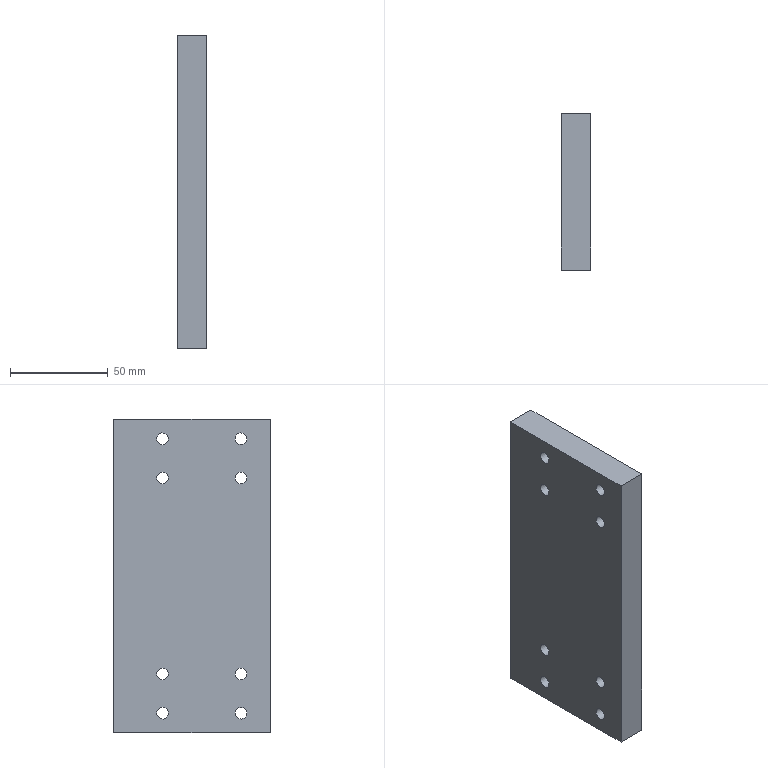Part | STEP file | SN10_008_007-01_PLACA | 1 solid | 14 faces | box 15 x 80 x 160 mm | volume 188607 mm3 | cylinder 8 | plane 6 | commonest cylinder face diameters 6 x8
STEP:
#1=CARTESIAN_POINT('',(0.,0.,0.));
#2=DIRECTION('',(0.,0.,1.));
#3=DIRECTION('',(1.,0.,0.));
#4=AXIS2_PLACEMENT_3D('',#1,#2,#3);
#5=CARTESIAN_POINT('',(308.629,177.633,427.708));
#6=VERTEX_POINT('',#5);
#7=CARTESIAN_POINT('',(308.629,175.,426.27));
#8=DIRECTION('',(1.,0.,0.));
#9=DIRECTION('',(0.,1.,0.));
#10=AXIS2_PLACEMENT_3D('',#7,#8,#9);
#11=CIRCLE('',#10,3.);
#12=CARTESIAN_POINT('',(308.729,175.,426.27));
#13=DIRECTION('',(1.,0.,0.));
#14=DIRECTION('',(0.,0.8776,0.4794));
#15=AXIS2_PLACEMENT_3D('',#12,#13,#14);
#16=CYLINDRICAL_SURFACE('',#15,3.);
#17=CARTESIAN_POINT('',(-0.5,-0.1));
#18=DIRECTION('',(1.,0.));
#19=VECTOR('',#18,1.);
#20=LINE('',#17,#19);
#21=(GEOMETRIC_REPRESENTATION_CONTEXT(2)PARAMETRIC_REPRESENTATION_CONTEXT()REPRESENTATION_CONTEXT('',''));
#22=DEFINITIONAL_REPRESENTATION('',(#20),#21);
#23=PCURVE('',#16,#22);
#24=CARTESIAN_POINT('',(308.629,240.,446.));
#25=DIRECTION('',(1.,0.,0.));
#26=DIRECTION('',(0.,0.,-1.));
#27=AXIS2_PLACEMENT_3D('',#24,#25,#26);
#28=PLANE('',#27);
#29=CARTESIAN_POINT('',(19.73,-65.));
#30=DIRECTION('',(0.,1.));
#31=AXIS2_PLACEMENT_2D('',#29,#30);
#32=CIRCLE('',#31,3.);
#33=(GEOMETRIC_REPRESENTATION_CONTEXT(2)PARAMETRIC_REPRESENTATION_CONTEXT()REPRESENTATION_CONTEXT('',''));
#34=DEFINITIONAL_REPRESENTATION('',(#32),#33);
#35=PCURVE('',#28,#34);
#36=SURFACE_CURVE('',#11,(#23,#35),.PCURVE_S1.);
#37=EDGE_CURVE('',#6,#6,#36,.T.);
#38=ORIENTED_EDGE('',*,*,#37,.T.);
#39=CARTESIAN_POINT('',(323.629,177.633,427.708));
#40=VERTEX_POINT('',#39);
#41=CARTESIAN_POINT('',(308.629,177.633,427.708));
#42=CARTESIAN_POINT('',(323.629,177.633,427.708));
#43=B_SPLINE_CURVE_WITH_KNOTS('',1,(#41,#42),.UNSPECIFIED.,.F.,.F.,(2,2),(-0.1,14.9),.PIECEWISE_BEZIER_KNOTS.);
#44=CARTESIAN_POINT('',(6.283,0.));
#45=DIRECTION('',(0.,1.));
#46=VECTOR('',#45,1.);
#47=LINE('',#44,#46);
#48=(GEOMETRIC_REPRESENTATION_CONTEXT(2)PARAMETRIC_REPRESENTATION_CONTEXT()REPRESENTATION_CONTEXT('',''));
#49=DEFINITIONAL_REPRESENTATION('',(#47),#48);
#50=PCURVE('',#16,#49);
#51=CARTESIAN_POINT('',(0.,0.));
#52=DIRECTION('',(0.,1.));
#53=VECTOR('',#52,1.);
#54=LINE('',#51,#53);
#55=(GEOMETRIC_REPRESENTATION_CONTEXT(2)PARAMETRIC_REPRESENTATION_CONTEXT()REPRESENTATION_CONTEXT('',''));
#56=DEFINITIONAL_REPRESENTATION('',(#54),#55);
#57=PCURVE('',#16,#56);
#58=SEAM_CURVE('',#43,(#50,#57),.PCURVE_S1.);
#59=EDGE_CURVE('',#6,#40,#58,.T.);
#60=ORIENTED_EDGE('',*,*,#59,.T.);
#61=CARTESIAN_POINT('',(323.629,175.,426.27));
#62=DIRECTION('',(1.,0.,0.));
#63=DIRECTION('',(0.,1.,0.));
#64=AXIS2_PLACEMENT_3D('',#61,#62,#63);
#65=CIRCLE('',#64,3.);
#66=CARTESIAN_POINT('',(-0.5,14.9));
#67=DIRECTION('',(1.,0.));
#68=VECTOR('',#67,1.);
#69=LINE('',#66,#68);
#70=(GEOMETRIC_REPRESENTATION_CONTEXT(2)PARAMETRIC_REPRESENTATION_CONTEXT()REPRESENTATION_CONTEXT('',''));
#71=DEFINITIONAL_REPRESENTATION('',(#69),#70);
#72=PCURVE('',#16,#71);
#73=CARTESIAN_POINT('',(323.629,160.,446.));
#74=DIRECTION('',(-1.,0.,0.));
#75=DIRECTION('',(0.,0.,1.));
#76=AXIS2_PLACEMENT_3D('',#73,#74,#75);
#77=PLANE('',#76);
#78=CARTESIAN_POINT('',(-19.73,18.));
#79=CARTESIAN_POINT('',(-14.533,18.));
#80=CARTESIAN_POINT('',(-17.131,13.5));
#81=CARTESIAN_POINT('',(-19.73,9.));
#82=CARTESIAN_POINT('',(-22.328,13.5));
#83=CARTESIAN_POINT('',(-24.926,18.));
#84=CARTESIAN_POINT('',(-19.73,18.));
#85=(BOUNDED_CURVE()B_SPLINE_CURVE(2,(#78,#79,#80,#81,#82,#83,#84),.UNSPECIFIED.,.T.,.F.)B_SPLINE_CURVE_WITH_KNOTS((1,2,2,2,2,1),(-2.094,0.,2.094,4.189,6.283,8.378),.UNSPECIFIED.)CURVE()GEOMETRIC_REPRESENTATION_ITEM()RATIONAL_B_SPLINE_CURVE((1.,0.5,1.,0.5,1.,0.5,1.))REPRESENTATION_ITEM(''));
#86=(GEOMETRIC_REPRESENTATION_CONTEXT(2)PARAMETRIC_REPRESENTATION_CONTEXT()REPRESENTATION_CONTEXT('',''));
#87=DEFINITIONAL_REPRESENTATION('',(#85),#86);
#88=PCURVE('',#77,#87);
#89=SURFACE_CURVE('',#65,(#72,#88),.PCURVE_S1.);
#90=EDGE_CURVE('',#40,#40,#89,.T.);
#91=ORIENTED_EDGE('',*,*,#90,.F.);
#92=ORIENTED_EDGE('',*,*,#59,.F.);
#93=EDGE_LOOP('',(#38,#60,#91,#92));
#94=FACE_BOUND('',#93,.F.);
#95=ADVANCED_FACE('',(#94),#16,.F.);
#96=CARTESIAN_POINT('',(308.629,160.,436.27));
#97=VERTEX_POINT('',#96);
#98=CARTESIAN_POINT('',(308.629,160.,276.27));
#99=VERTEX_POINT('',#98);
#100=CARTESIAN_POINT('',(308.629,160.,436.27));
#101=DIRECTION('',(0.,0.,-1.));
#102=VECTOR('',#101,1.);
#103=LINE('',#100,#102);
#104=CARTESIAN_POINT('',(323.629,160.,446.));
#105=DIRECTION('',(0.,-1.,0.));
#106=DIRECTION('',(0.,0.,-1.));
#107=AXIS2_PLACEMENT_3D('',#104,#105,#106);
#108=PLANE('',#107);
#109=CARTESIAN_POINT('',(9.73,-15.));
#110=DIRECTION('',(1.,0.));
#111=VECTOR('',#110,1.);
#112=LINE('',#109,#111);
#113=(GEOMETRIC_REPRESENTATION_CONTEXT(2)PARAMETRIC_REPRESENTATION_CONTEXT()REPRESENTATION_CONTEXT('',''));
#114=DEFINITIONAL_REPRESENTATION('',(#112),#113);
#115=PCURVE('',#108,#114);
#116=CARTESIAN_POINT('',(9.73,-80.));
#117=DIRECTION('',(1.,0.));
#118=VECTOR('',#117,1.);
#119=LINE('',#116,#118);
#120=(GEOMETRIC_REPRESENTATION_CONTEXT(2)PARAMETRIC_REPRESENTATION_CONTEXT()REPRESENTATION_CONTEXT('',''));
#121=DEFINITIONAL_REPRESENTATION('',(#119),#120);
#122=PCURVE('',#28,#121);
#123=SURFACE_CURVE('',#103,(#115,#122),.PCURVE_S1.);
#124=EDGE_CURVE('',#97,#99,#123,.T.);
#125=ORIENTED_EDGE('',*,*,#124,.T.);
#126=CARTESIAN_POINT('',(323.629,160.,276.27));
#127=VERTEX_POINT('',#126);
#128=CARTESIAN_POINT('',(323.629,160.,276.27));
#129=DIRECTION('',(-1.,0.,0.));
#130=VECTOR('',#129,1.);
#131=LINE('',#128,#130);
#132=CARTESIAN_POINT('',(169.73,0.));
#133=DIRECTION('',(0.,-1.));
#134=VECTOR('',#133,1.);
#135=LINE('',#132,#134);
#136=(GEOMETRIC_REPRESENTATION_CONTEXT(2)PARAMETRIC_REPRESENTATION_CONTEXT()REPRESENTATION_CONTEXT('',''));
#137=DEFINITIONAL_REPRESENTATION('',(#135),#136);
#138=PCURVE('',#108,#137);
#139=CARTESIAN_POINT('',(243.629,270.,276.27));
#140=DIRECTION('',(0.,0.,-1.));
#141=DIRECTION('',(-1.,0.,0.));
#142=AXIS2_PLACEMENT_3D('',#139,#140,#141);
#143=PLANE('',#142);
#144=CARTESIAN_POINT('',(-80.,-110.));
#145=DIRECTION('',(1.,0.));
#146=VECTOR('',#145,1.);
#147=LINE('',#144,#146);
#148=(GEOMETRIC_REPRESENTATION_CONTEXT(2)PARAMETRIC_REPRESENTATION_CONTEXT()REPRESENTATION_CONTEXT('',''));
#149=DEFINITIONAL_REPRESENTATION('',(#147),#148);
#150=PCURVE('',#143,#149);
#151=SURFACE_CURVE('',#131,(#138,#150),.PCURVE_S1.);
#152=EDGE_CURVE('',#127,#99,#151,.T.);
#153=ORIENTED_EDGE('',*,*,#152,.F.);
#154=CARTESIAN_POINT('',(323.629,160.,436.27));
#155=VERTEX_POINT('',#154);
#156=CARTESIAN_POINT('',(323.629,160.,436.27));
#157=DIRECTION('',(0.,0.,-1.));
#158=VECTOR('',#157,1.);
#159=LINE('',#156,#158);
#160=CARTESIAN_POINT('',(9.73,0.));
#161=DIRECTION('',(1.,0.));
#162=VECTOR('',#161,1.);
#163=LINE('',#160,#162);
#164=(GEOMETRIC_REPRESENTATION_CONTEXT(2)PARAMETRIC_REPRESENTATION_CONTEXT()REPRESENTATION_CONTEXT('',''));
#165=DEFINITIONAL_REPRESENTATION('',(#163),#164);
#166=PCURVE('',#108,#165);
#167=CARTESIAN_POINT('',(-9.73,0.));
#168=DIRECTION('',(-1.,0.));
#169=VECTOR('',#168,1.);
#170=LINE('',#167,#169);
#171=(GEOMETRIC_REPRESENTATION_CONTEXT(2)PARAMETRIC_REPRESENTATION_CONTEXT()REPRESENTATION_CONTEXT('',''));
#172=DEFINITIONAL_REPRESENTATION('',(#170),#171);
#173=PCURVE('',#77,#172);
#174=SURFACE_CURVE('',#159,(#166,#173),.PCURVE_S1.);
#175=EDGE_CURVE('',#155,#127,#174,.T.);
#176=ORIENTED_EDGE('',*,*,#175,.F.);
#177=CARTESIAN_POINT('',(308.629,160.,436.27));
#178=DIRECTION('',(1.,0.,0.));
#179=VECTOR('',#178,1.);
#180=LINE('',#177,#179);
#181=CARTESIAN_POINT('',(9.73,-15.));
#182=DIRECTION('',(0.,1.));
#183=VECTOR('',#182,1.);
#184=LINE('',#181,#183);
#185=(GEOMETRIC_REPRESENTATION_CONTEXT(2)PARAMETRIC_REPRESENTATION_CONTEXT()REPRESENTATION_CONTEXT('',''));
#186=DEFINITIONAL_REPRESENTATION('',(#184),#185);
#187=PCURVE('',#108,#186);
#188=CARTESIAN_POINT('',(308.629,245.913,436.27));
#189=DIRECTION('',(0.,0.,-1.));
#190=DIRECTION('',(-1.,0.,0.));
#191=AXIS2_PLACEMENT_3D('',#188,#189,#190);
#192=PLANE('',#191);
#193=CARTESIAN_POINT('',(0.,-85.913));
#194=DIRECTION('',(-1.,0.));
#195=VECTOR('',#194,1.);
#196=LINE('',#193,#195);
#197=(GEOMETRIC_REPRESENTATION_CONTEXT(2)PARAMETRIC_REPRESENTATION_CONTEXT()REPRESENTATION_CONTEXT('',''));
#198=DEFINITIONAL_REPRESENTATION('',(#196),#197);
#199=PCURVE('',#192,#198);
#200=SURFACE_CURVE('',#180,(#187,#199),.PCURVE_S1.);
#201=EDGE_CURVE('',#97,#155,#200,.T.);
#202=ORIENTED_EDGE('',*,*,#201,.F.);
#203=EDGE_LOOP('',(#125,#153,#176,#202));
#204=FACE_BOUND('',#203,.T.);
#205=ADVANCED_FACE('',(#204),#108,.T.);
#206=CARTESIAN_POINT('',(323.629,240.,276.27));
#207=VERTEX_POINT('',#206);
#208=CARTESIAN_POINT('',(323.629,160.,276.27));
#209=DIRECTION('',(0.,1.,0.));
#210=VECTOR('',#209,1.);
#211=LINE('',#208,#210);
#212=CARTESIAN_POINT('',(-80.,-110.));
#213=DIRECTION('',(0.,1.));
#214=VECTOR('',#213,1.);
#215=LINE('',#212,#214);
#216=(GEOMETRIC_REPRESENTATION_CONTEXT(2)PARAMETRIC_REPRESENTATION_CONTEXT()REPRESENTATION_CONTEXT('',''));
#217=DEFINITIONAL_REPRESENTATION('',(#215),#216);
#218=PCURVE('',#143,#217);
#219=CARTESIAN_POINT('',(-169.73,0.));
#220=DIRECTION('',(0.,1.));
#221=VECTOR('',#220,1.);
#222=LINE('',#219,#221);
#223=(GEOMETRIC_REPRESENTATION_CONTEXT(2)PARAMETRIC_REPRESENTATION_CONTEXT()REPRESENTATION_CONTEXT('',''));
#224=DEFINITIONAL_REPRESENTATION('',(#222),#223);
#225=PCURVE('',#77,#224);
#226=SURFACE_CURVE('',#211,(#218,#225),.PCURVE_S1.);
#227=EDGE_CURVE('',#127,#207,#226,.T.);
#228=ORIENTED_EDGE('',*,*,#227,.F.);
#229=ORIENTED_EDGE('',*,*,#152,.T.);
#230=CARTESIAN_POINT('',(308.629,240.,276.27));
#231=VERTEX_POINT('',#230);
#232=CARTESIAN_POINT('',(308.629,240.,276.27));
#233=DIRECTION('',(0.,-1.,0.));
#234=VECTOR('',#233,1.);
#235=LINE('',#232,#234);
#236=CARTESIAN_POINT('',(-65.,-30.));
#237=DIRECTION('',(0.,-1.));
#238=VECTOR('',#237,1.);
#239=LINE('',#236,#238);
#240=(GEOMETRIC_REPRESENTATION_CONTEXT(2)PARAMETRIC_REPRESENTATION_CONTEXT()REPRESENTATION_CONTEXT('',''));
#241=DEFINITIONAL_REPRESENTATION('',(#239),#240);
#242=PCURVE('',#143,#241);
#243=CARTESIAN_POINT('',(169.73,0.));
#244=DIRECTION('',(0.,-1.));
#245=VECTOR('',#244,1.);
#246=LINE('',#243,#245);
#247=(GEOMETRIC_REPRESENTATION_CONTEXT(2)PARAMETRIC_REPRESENTATION_CONTEXT()REPRESENTATION_CONTEXT('',''));
#248=DEFINITIONAL_REPRESENTATION('',(#246),#247);
#249=PCURVE('',#28,#248);
#250=SURFACE_CURVE('',#235,(#242,#249),.PCURVE_S1.);
#251=EDGE_CURVE('',#231,#99,#250,.T.);
#252=ORIENTED_EDGE('',*,*,#251,.F.);
#253=CARTESIAN_POINT('',(308.629,240.,276.27));
#254=DIRECTION('',(1.,0.,0.));
#255=VECTOR('',#254,1.);
#256=LINE('',#253,#255);
#257=CARTESIAN_POINT('',(-65.,-30.));
#258=DIRECTION('',(-1.,0.));
#259=VECTOR('',#258,1.);
#260=LINE('',#257,#259);
#261=(GEOMETRIC_REPRESENTATION_CONTEXT(2)PARAMETRIC_REPRESENTATION_CONTEXT()REPRESENTATION_CONTEXT('',''));
#262=DEFINITIONAL_REPRESENTATION('',(#260),#261);
#263=PCURVE('',#143,#262);
#264=CARTESIAN_POINT('',(308.629,240.,446.));
#265=DIRECTION('',(0.,1.,0.));
#266=DIRECTION('',(0.,0.,1.));
#267=AXIS2_PLACEMENT_3D('',#264,#265,#266);
#268=PLANE('',#267);
#269=CARTESIAN_POINT('',(-169.73,0.));
#270=DIRECTION('',(0.,1.));
#271=VECTOR('',#270,1.);
#272=LINE('',#269,#271);
#273=(GEOMETRIC_REPRESENTATION_CONTEXT(2)PARAMETRIC_REPRESENTATION_CONTEXT()REPRESENTATION_CONTEXT('',''));
#274=DEFINITIONAL_REPRESENTATION('',(#272),#273);
#275=PCURVE('',#268,#274);
#276=SURFACE_CURVE('',#256,(#263,#275),.PCURVE_S1.);
#277=EDGE_CURVE('',#231,#207,#276,.T.);
#278=ORIENTED_EDGE('',*,*,#277,.T.);
#279=EDGE_LOOP('',(#228,#229,#252,#278));
#280=FACE_BOUND('',#279,.T.);
#281=ADVANCED_FACE('',(#280),#143,.T.);
#282=CARTESIAN_POINT('',(323.629,240.,436.27));
#283=VERTEX_POINT('',#282);
#284=CARTESIAN_POINT('',(323.629,240.,436.27));
#285=DIRECTION('',(0.,0.,-1.));
#286=VECTOR('',#285,1.);
#287=LINE('',#284,#286);
#288=CARTESIAN_POINT('',(-9.73,15.));
#289=DIRECTION('',(-1.,0.));
#290=VECTOR('',#289,1.);
#291=LINE('',#288,#290);
#292=(GEOMETRIC_REPRESENTATION_CONTEXT(2)PARAMETRIC_REPRESENTATION_CONTEXT()REPRESENTATION_CONTEXT('',''));
#293=DEFINITIONAL_REPRESENTATION('',(#291),#292);
#294=PCURVE('',#268,#293);
#295=CARTESIAN_POINT('',(-9.73,80.));
#296=DIRECTION('',(-1.,0.));
#297=VECTOR('',#296,1.);
#298=LINE('',#295,#297);
#299=(GEOMETRIC_REPRESENTATION_CONTEXT(2)PARAMETRIC_REPRESENTATION_CONTEXT()REPRESENTATION_CONTEXT('',''));
#300=DEFINITIONAL_REPRESENTATION('',(#298),#299);
#301=PCURVE('',#77,#300);
#302=SURFACE_CURVE('',#287,(#294,#301),.PCURVE_S1.);
#303=EDGE_CURVE('',#283,#207,#302,.T.);
#304=ORIENTED_EDGE('',*,*,#303,.T.);
#305=ORIENTED_EDGE('',*,*,#277,.F.);
#306=CARTESIAN_POINT('',(308.629,240.,436.27));
#307=VERTEX_POINT('',#306);
#308=CARTESIAN_POINT('',(308.629,240.,436.27));
#309=DIRECTION('',(0.,0.,-1.));
#310=VECTOR('',#309,1.);
#311=LINE('',#308,#310);
#312=CARTESIAN_POINT('',(-9.73,0.));
#313=DIRECTION('',(-1.,0.));
#314=VECTOR('',#313,1.);
#315=LINE('',#312,#314);
#316=(GEOMETRIC_REPRESENTATION_CONTEXT(2)PARAMETRIC_REPRESENTATION_CONTEXT()REPRESENTATION_CONTEXT('',''));
#317=DEFINITIONAL_REPRESENTATION('',(#315),#316);
#318=PCURVE('',#268,#317);
#319=CARTESIAN_POINT('',(9.73,0.));
#320=DIRECTION('',(1.,0.));
#321=VECTOR('',#320,1.);
#322=LINE('',#319,#321);
#323=(GEOMETRIC_REPRESENTATION_CONTEXT(2)PARAMETRIC_REPRESENTATION_CONTEXT()REPRESENTATION_CONTEXT('',''));
#324=DEFINITIONAL_REPRESENTATION('',(#322),#323);
#325=PCURVE('',#28,#324);
#326=SURFACE_CURVE('',#311,(#318,#325),.PCURVE_S1.);
#327=EDGE_CURVE('',#307,#231,#326,.T.);
#328=ORIENTED_EDGE('',*,*,#327,.F.);
#329=CARTESIAN_POINT('',(308.629,240.,436.27));
#330=DIRECTION('',(1.,0.,0.));
#331=VECTOR('',#330,1.);
#332=LINE('',#329,#331);
#333=CARTESIAN_POINT('',(-9.73,0.));
#334=DIRECTION('',(0.,1.));
#335=VECTOR('',#334,1.);
#336=LINE('',#333,#335);
#337=(GEOMETRIC_REPRESENTATION_CONTEXT(2)PARAMETRIC_REPRESENTATION_CONTEXT()REPRESENTATION_CONTEXT('',''));
#338=DEFINITIONAL_REPRESENTATION('',(#336),#337);
#339=PCURVE('',#268,#338);
#340=CARTESIAN_POINT('',(0.,-5.913));
#341=DIRECTION('',(-1.,0.));
#342=VECTOR('',#341,1.);
#343=LINE('',#340,#342);
#344=(GEOMETRIC_REPRESENTATION_CONTEXT(2)PARAMETRIC_REPRESENTATION_CONTEXT()REPRESENTATION_CONTEXT('',''));
#345=DEFINITIONAL_REPRESENTATION('',(#343),#344);
#346=PCURVE('',#192,#345);
#347=SURFACE_CURVE('',#332,(#339,#346),.PCURVE_S1.);
#348=EDGE_CURVE('',#307,#283,#347,.T.);
#349=ORIENTED_EDGE('',*,*,#348,.T.);
#350=EDGE_LOOP('',(#304,#305,#328,#349));
#351=FACE_BOUND('',#350,.T.);
#352=ADVANCED_FACE('',(#351),#268,.T.);
#353=ORIENTED_EDGE('',*,*,#201,.T.);
#354=CARTESIAN_POINT('',(323.629,160.,436.27));
#355=DIRECTION('',(0.,1.,0.));
#356=VECTOR('',#355,1.);
#357=LINE('',#354,#356);
#358=CARTESIAN_POINT('',(-15.,-85.913));
#359=DIRECTION('',(0.,1.));
#360=VECTOR('',#359,1.);
#361=LINE('',#358,#360);
#362=(GEOMETRIC_REPRESENTATION_CONTEXT(2)PARAMETRIC_REPRESENTATION_CONTEXT()REPRESENTATION_CONTEXT('',''));
#363=DEFINITIONAL_REPRESENTATION('',(#361),#362);
#364=PCURVE('',#192,#363);
#365=CARTESIAN_POINT('',(-9.73,0.));
#366=DIRECTION('',(0.,1.));
#367=VECTOR('',#366,1.);
#368=LINE('',#365,#367);
#369=(GEOMETRIC_REPRESENTATION_CONTEXT(2)PARAMETRIC_REPRESENTATION_CONTEXT()REPRESENTATION_CONTEXT('',''));
#370=DEFINITIONAL_REPRESENTATION('',(#368),#369);
#371=PCURVE('',#77,#370);
#372=SURFACE_CURVE('',#357,(#364,#371),.PCURVE_S1.);
#373=EDGE_CURVE('',#155,#283,#372,.T.);
#374=ORIENTED_EDGE('',*,*,#373,.T.);
#375=ORIENTED_EDGE('',*,*,#348,.F.);
#376=CARTESIAN_POINT('',(308.629,240.,436.27));
#377=DIRECTION('',(0.,-1.,0.));
#378=VECTOR('',#377,1.);
#379=LINE('',#376,#378);
#380=CARTESIAN_POINT('',(0.,-5.913));
#381=DIRECTION('',(0.,-1.));
#382=VECTOR('',#381,1.);
#383=LINE('',#380,#382);
#384=(GEOMETRIC_REPRESENTATION_CONTEXT(2)PARAMETRIC_REPRESENTATION_CONTEXT()REPRESENTATION_CONTEXT('',''));
#385=DEFINITIONAL_REPRESENTATION('',(#383),#384);
#386=PCURVE('',#192,#385);
#387=CARTESIAN_POINT('',(9.73,0.));
#388=DIRECTION('',(0.,-1.));
#389=VECTOR('',#388,1.);
#390=LINE('',#387,#389);
#391=(GEOMETRIC_REPRESENTATION_CONTEXT(2)PARAMETRIC_REPRESENTATION_CONTEXT()REPRESENTATION_CONTEXT('',''));
#392=DEFINITIONAL_REPRESENTATION('',(#390),#391);
#393=PCURVE('',#28,#392);
#394=SURFACE_CURVE('',#379,(#386,#393),.PCURVE_S1.);
#395=EDGE_CURVE('',#307,#97,#394,.T.);
#396=ORIENTED_EDGE('',*,*,#395,.T.);
#397=EDGE_LOOP('',(#353,#374,#375,#396));
#398=FACE_BOUND('',#397,.T.);
#399=ADVANCED_FACE('',(#398),#192,.F.);
#400=CARTESIAN_POINT('',(308.629,217.633,427.708));
#401=VERTEX_POINT('',#400);
#402=CARTESIAN_POINT('',(308.629,215.,426.27));
#403=DIRECTION('',(1.,0.,0.));
#404=DIRECTION('',(0.,1.,0.));
#405=AXIS2_PLACEMENT_3D('',#402,#403,#404);
#406=CIRCLE('',#405,3.);
#407=CARTESIAN_POINT('',(308.729,215.,426.27));
#408=DIRECTION('',(1.,0.,0.));
#409=DIRECTION('',(0.,0.8776,0.4794));
#410=AXIS2_PLACEMENT_3D('',#407,#408,#409);
#411=CYLINDRICAL_SURFACE('',#410,3.);
#412=CARTESIAN_POINT('',(-0.5,-0.1));
#413=DIRECTION('',(1.,0.));
#414=VECTOR('',#413,1.);
#415=LINE('',#412,#414);
#416=(GEOMETRIC_REPRESENTATION_CONTEXT(2)PARAMETRIC_REPRESENTATION_CONTEXT()REPRESENTATION_CONTEXT('',''));
#417=DEFINITIONAL_REPRESENTATION('',(#415),#416);
#418=PCURVE('',#411,#417);
#419=CARTESIAN_POINT('',(19.73,-25.));
#420=DIRECTION('',(0.,1.));
#421=AXIS2_PLACEMENT_2D('',#419,#420);
#422=CIRCLE('',#421,3.);
#423=(GEOMETRIC_REPRESENTATION_CONTEXT(2)PARAMETRIC_REPRESENTATION_CONTEXT()REPRESENTATION_CONTEXT('',''));
#424=DEFINITIONAL_REPRESENTATION('',(#422),#423);
#425=PCURVE('',#28,#424);
#426=SURFACE_CURVE('',#406,(#418,#425),.PCURVE_S1.);
#427=EDGE_CURVE('',#401,#401,#426,.T.);
#428=ORIENTED_EDGE('',*,*,#427,.T.);
#429=CARTESIAN_POINT('',(323.629,217.633,427.708));
#430=VERTEX_POINT('',#429);
#431=CARTESIAN_POINT('',(308.629,217.633,427.708));
#432=CARTESIAN_POINT('',(323.629,217.633,427.708));
#433=B_SPLINE_CURVE_WITH_KNOTS('',1,(#431,#432),.UNSPECIFIED.,.F.,.F.,(2,2),(-0.1,14.9),.PIECEWISE_BEZIER_KNOTS.);
#434=CARTESIAN_POINT('',(6.283,0.));
#435=DIRECTION('',(0.,1.));
#436=VECTOR('',#435,1.);
#437=LINE('',#434,#436);
#438=(GEOMETRIC_REPRESENTATION_CONTEXT(2)PARAMETRIC_REPRESENTATION_CONTEXT()REPRESENTATION_CONTEXT('',''));
#439=DEFINITIONAL_REPRESENTATION('',(#437),#438);
#440=PCURVE('',#411,#439);
#441=CARTESIAN_POINT('',(0.,0.));
#442=DIRECTION('',(0.,1.));
#443=VECTOR('',#442,1.);
#444=LINE('',#441,#443);
#445=(GEOMETRIC_REPRESENTATION_CONTEXT(2)PARAMETRIC_REPRESENTATION_CONTEXT()REPRESENTATION_CONTEXT('',''));
#446=DEFINITIONAL_REPRESENTATION('',(#444),#445);
#447=PCURVE('',#411,#446);
#448=SEAM_CURVE('',#433,(#440,#447),.PCURVE_S1.);
#449=EDGE_CURVE('',#401,#430,#448,.T.);
#450=ORIENTED_EDGE('',*,*,#449,.T.);
#451=CARTESIAN_POINT('',(323.629,215.,426.27));
#452=DIRECTION('',(1.,0.,0.));
#453=DIRECTION('',(0.,1.,0.));
#454=AXIS2_PLACEMENT_3D('',#451,#452,#453);
#455=CIRCLE('',#454,3.);
#456=CARTESIAN_POINT('',(-0.5,14.9));
#457=DIRECTION('',(1.,0.));
#458=VECTOR('',#457,1.);
#459=LINE('',#456,#458);
#460=(GEOMETRIC_REPRESENTATION_CONTEXT(2)PARAMETRIC_REPRESENTATION_CONTEXT()REPRESENTATION_CONTEXT('',''));
#461=DEFINITIONAL_REPRESENTATION('',(#459),#460);
#462=PCURVE('',#411,#461);
#463=CARTESIAN_POINT('',(-19.73,58.));
#464=CARTESIAN_POINT('',(-14.533,58.));
#465=CARTESIAN_POINT('',(-17.131,53.5));
#466=CARTESIAN_POINT('',(-19.73,49.));
#467=CARTESIAN_POINT('',(-22.328,53.5));
#468=CARTESIAN_POINT('',(-24.926,58.));
#469=CARTESIAN_POINT('',(-19.73,58.));
#470=(BOUNDED_CURVE()B_SPLINE_CURVE(2,(#463,#464,#465,#466,#467,#468,#469),.UNSPECIFIED.,.T.,.F.)B_SPLINE_CURVE_WITH_KNOTS((1,2,2,2,2,1),(-2.094,0.,2.094,4.189,6.283,8.378),.UNSPECIFIED.)CURVE()GEOMETRIC_REPRESENTATION_ITEM()RATIONAL_B_SPLINE_CURVE((1.,0.5,1.,0.5,1.,0.5,1.))REPRESENTATION_ITEM(''));
#471=(GEOMETRIC_REPRESENTATION_CONTEXT(2)PARAMETRIC_REPRESENTATION_CONTEXT()REPRESENTATION_CONTEXT('',''));
#472=DEFINITIONAL_REPRESENTATION('',(#470),#471);
#473=PCURVE('',#77,#472);
#474=SURFACE_CURVE('',#455,(#462,#473),.PCURVE_S1.);
#475=EDGE_CURVE('',#430,#430,#474,.T.);
#476=ORIENTED_EDGE('',*,*,#475,.F.);
#477=ORIENTED_EDGE('',*,*,#449,.F.);
#478=EDGE_LOOP('',(#428,#450,#476,#477));
#479=FACE_BOUND('',#478,.F.);
#480=ADVANCED_FACE('',(#479),#411,.F.);
#481=CARTESIAN_POINT('',(308.629,177.633,407.708));
#482=VERTEX_POINT('',#481);
#483=CARTESIAN_POINT('',(308.629,175.,406.27));
#484=DIRECTION('',(1.,0.,0.));
#485=DIRECTION('',(0.,1.,0.));
#486=AXIS2_PLACEMENT_3D('',#483,#484,#485);
#487=CIRCLE('',#486,3.);
#488=CARTESIAN_POINT('',(308.729,175.,406.27));
#489=DIRECTION('',(1.,0.,0.));
#490=DIRECTION('',(0.,0.8776,0.4794));
#491=AXIS2_PLACEMENT_3D('',#488,#489,#490);
#492=CYLINDRICAL_SURFACE('',#491,3.);
#493=CARTESIAN_POINT('',(-0.5,-0.1));
#494=DIRECTION('',(1.,0.));
#495=VECTOR('',#494,1.);
#496=LINE('',#493,#495);
#497=(GEOMETRIC_REPRESENTATION_CONTEXT(2)PARAMETRIC_REPRESENTATION_CONTEXT()REPRESENTATION_CONTEXT('',''));
#498=DEFINITIONAL_REPRESENTATION('',(#496),#497);
#499=PCURVE('',#492,#498);
#500=CARTESIAN_POINT('',(39.73,-65.));
#501=DIRECTION('',(0.,1.));
#502=AXIS2_PLACEMENT_2D('',#500,#501);
#503=CIRCLE('',#502,3.);
#504=(GEOMETRIC_REPRESENTATION_CONTEXT(2)PARAMETRIC_REPRESENTATION_CONTEXT()REPRESENTATION_CONTEXT('',''));
#505=DEFINITIONAL_REPRESENTATION('',(#503),#504);
#506=PCURVE('',#28,#505);
#507=SURFACE_CURVE('',#487,(#499,#506),.PCURVE_S1.);
#508=EDGE_CURVE('',#482,#482,#507,.T.);
#509=ORIENTED_EDGE('',*,*,#508,.T.);
#510=CARTESIAN_POINT('',(323.629,177.633,407.708));
#511=VERTEX_POINT('',#510);
#512=CARTESIAN_POINT('',(308.629,177.633,407.708));
#513=CARTESIAN_POINT('',(323.629,177.633,407.708));
#514=B_SPLINE_CURVE_WITH_KNOTS('',1,(#512,#513),.UNSPECIFIED.,.F.,.F.,(2,2),(-0.1,14.9),.PIECEWISE_BEZIER_KNOTS.);
#515=CARTESIAN_POINT('',(6.283,0.));
#516=DIRECTION('',(0.,1.));
#517=VECTOR('',#516,1.);
#518=LINE('',#515,#517);
#519=(GEOMETRIC_REPRESENTATION_CONTEXT(2)PARAMETRIC_REPRESENTATION_CONTEXT()REPRESENTATION_CONTEXT('',''));
#520=DEFINITIONAL_REPRESENTATION('',(#518),#519);
#521=PCURVE('',#492,#520);
#522=CARTESIAN_POINT('',(0.,0.));
#523=DIRECTION('',(0.,1.));
#524=VECTOR('',#523,1.);
#525=LINE('',#522,#524);
#526=(GEOMETRIC_REPRESENTATION_CONTEXT(2)PARAMETRIC_REPRESENTATION_CONTEXT()REPRESENTATION_CONTEXT('',''));
#527=DEFINITIONAL_REPRESENTATION('',(#525),#526);
#528=PCURVE('',#492,#527);
#529=SEAM_CURVE('',#514,(#521,#528),.PCURVE_S1.);
#530=EDGE_CURVE('',#482,#511,#529,.T.);
#531=ORIENTED_EDGE('',*,*,#530,.T.);
#532=CARTESIAN_POINT('',(323.629,175.,406.27));
#533=DIRECTION('',(1.,0.,0.));
#534=DIRECTION('',(0.,1.,0.));
#535=AXIS2_PLACEMENT_3D('',#532,#533,#534);
#536=CIRCLE('',#535,3.);
#537=CARTESIAN_POINT('',(-0.5,14.9));
#538=DIRECTION('',(1.,0.));
#539=VECTOR('',#538,1.);
#540=LINE('',#537,#539);
#541=(GEOMETRIC_REPRESENTATION_CONTEXT(2)PARAMETRIC_REPRESENTATION_CONTEXT()REPRESENTATION_CONTEXT('',''));
#542=DEFINITIONAL_REPRESENTATION('',(#540),#541);
#543=PCURVE('',#492,#542);
#544=CARTESIAN_POINT('',(-39.73,18.));
#545=CARTESIAN_POINT('',(-34.533,18.));
#546=CARTESIAN_POINT('',(-37.131,13.5));
#547=CARTESIAN_POINT('',(-39.73,9.));
#548=CARTESIAN_POINT('',(-42.328,13.5));
#549=CARTESIAN_POINT('',(-44.926,18.));
#550=CARTESIAN_POINT('',(-39.73,18.));
#551=(BOUNDED_CURVE()B_SPLINE_CURVE(2,(#544,#545,#546,#547,#548,#549,#550),.UNSPECIFIED.,.T.,.F.)B_SPLINE_CURVE_WITH_KNOTS((1,2,2,2,2,1),(-2.094,0.,2.094,4.189,6.283,8.378),.UNSPECIFIED.)CURVE()GEOMETRIC_REPRESENTATION_ITEM()RATIONAL_B_SPLINE_CURVE((1.,0.5,1.,0.5,1.,0.5,1.))REPRESENTATION_ITEM(''));
#552=(GEOMETRIC_REPRESENTATION_CONTEXT(2)PARAMETRIC_REPRESENTATION_CONTEXT()REPRESENTATION_CONTEXT('',''));
#553=DEFINITIONAL_REPRESENTATION('',(#551),#552);
#554=PCURVE('',#77,#553);
#555=SURFACE_CURVE('',#536,(#543,#554),.PCURVE_S1.);
#556=EDGE_CURVE('',#511,#511,#555,.T.);
#557=ORIENTED_EDGE('',*,*,#556,.F.);
#558=ORIENTED_EDGE('',*,*,#530,.F.);
#559=EDGE_LOOP('',(#509,#531,#557,#558));
#560=FACE_BOUND('',#559,.F.);
#561=ADVANCED_FACE('',(#560),#492,.F.);
#562=CARTESIAN_POINT('',(308.629,217.633,407.708));
#563=VERTEX_POINT('',#562);
#564=CARTESIAN_POINT('',(308.629,215.,406.27));
#565=DIRECTION('',(1.,0.,0.));
#566=DIRECTION('',(0.,1.,0.));
#567=AXIS2_PLACEMENT_3D('',#564,#565,#566);
#568=CIRCLE('',#567,3.);
#569=CARTESIAN_POINT('',(308.729,215.,406.27));
#570=DIRECTION('',(1.,0.,0.));
#571=DIRECTION('',(0.,0.8776,0.4794));
#572=AXIS2_PLACEMENT_3D('',#569,#570,#571);
#573=CYLINDRICAL_SURFACE('',#572,3.);
#574=CARTESIAN_POINT('',(-0.5,-0.1));
#575=DIRECTION('',(1.,0.));
#576=VECTOR('',#575,1.);
#577=LINE('',#574,#576);
#578=(GEOMETRIC_REPRESENTATION_CONTEXT(2)PARAMETRIC_REPRESENTATION_CONTEXT()REPRESENTATION_CONTEXT('',''));
#579=DEFINITIONAL_REPRESENTATION('',(#577),#578);
#580=PCURVE('',#573,#579);
#581=CARTESIAN_POINT('',(39.73,-25.));
#582=DIRECTION('',(0.,1.));
#583=AXIS2_PLACEMENT_2D('',#581,#582);
#584=CIRCLE('',#583,3.);
#585=(GEOMETRIC_REPRESENTATION_CONTEXT(2)PARAMETRIC_REPRESENTATION_CONTEXT()REPRESENTATION_CONTEXT('',''));
#586=DEFINITIONAL_REPRESENTATION('',(#584),#585);
#587=PCURVE('',#28,#586);
#588=SURFACE_CURVE('',#568,(#580,#587),.PCURVE_S1.);
#589=EDGE_CURVE('',#563,#563,#588,.T.);
#590=ORIENTED_EDGE('',*,*,#589,.T.);
#591=CARTESIAN_POINT('',(323.629,217.633,407.708));
#592=VERTEX_POINT('',#591);
#593=CARTESIAN_POINT('',(308.629,217.633,407.708));
#594=CARTESIAN_POINT('',(323.629,217.633,407.708));
#595=B_SPLINE_CURVE_WITH_KNOTS('',1,(#593,#594),.UNSPECIFIED.,.F.,.F.,(2,2),(-0.1,14.9),.PIECEWISE_BEZIER_KNOTS.);
#596=CARTESIAN_POINT('',(6.283,0.));
#597=DIRECTION('',(0.,1.));
#598=VECTOR('',#597,1.);
#599=LINE('',#596,#598);
#600=(GEOMETRIC_REPRESENTATION_CONTEXT(2)PARAMETRIC_REPRESENTATION_CONTEXT()REPRESENTATION_CONTEXT('',''));
#601=DEFINITIONAL_REPRESENTATION('',(#599),#600);
#602=PCURVE('',#573,#601);
#603=CARTESIAN_POINT('',(0.,0.));
#604=DIRECTION('',(0.,1.));
#605=VECTOR('',#604,1.);
#606=LINE('',#603,#605);
#607=(GEOMETRIC_REPRESENTATION_CONTEXT(2)PARAMETRIC_REPRESENTATION_CONTEXT()REPRESENTATION_CONTEXT('',''));
#608=DEFINITIONAL_REPRESENTATION('',(#606),#607);
#609=PCURVE('',#573,#608);
#610=SEAM_CURVE('',#595,(#602,#609),.PCURVE_S1.);
#611=EDGE_CURVE('',#563,#592,#610,.T.);
#612=ORIENTED_EDGE('',*,*,#611,.T.);
#613=CARTESIAN_POINT('',(323.629,215.,406.27));
#614=DIRECTION('',(1.,0.,0.));
#615=DIRECTION('',(0.,1.,0.));
#616=AXIS2_PLACEMENT_3D('',#613,#614,#615);
#617=CIRCLE('',#616,3.);
#618=CARTESIAN_POINT('',(-0.5,14.9));
#619=DIRECTION('',(1.,0.));
#620=VECTOR('',#619,1.);
#621=LINE('',#618,#620);
#622=(GEOMETRIC_REPRESENTATION_CONTEXT(2)PARAMETRIC_REPRESENTATION_CONTEXT()REPRESENTATION_CONTEXT('',''));
#623=DEFINITIONAL_REPRESENTATION('',(#621),#622);
#624=PCURVE('',#573,#623);
#625=CARTESIAN_POINT('',(-39.73,58.));
#626=CARTESIAN_POINT('',(-34.533,58.));
#627=CARTESIAN_POINT('',(-37.131,53.5));
#628=CARTESIAN_POINT('',(-39.73,49.));
#629=CARTESIAN_POINT('',(-42.328,53.5));
#630=CARTESIAN_POINT('',(-44.926,58.));
#631=CARTESIAN_POINT('',(-39.73,58.));
#632=(BOUNDED_CURVE()B_SPLINE_CURVE(2,(#625,#626,#627,#628,#629,#630,#631),.UNSPECIFIED.,.T.,.F.)B_SPLINE_CURVE_WITH_KNOTS((1,2,2,2,2,1),(-2.094,0.,2.094,4.189,6.283,8.378),.UNSPECIFIED.)CURVE()GEOMETRIC_REPRESENTATION_ITEM()RATIONAL_B_SPLINE_CURVE((1.,0.5,1.,0.5,1.,0.5,1.))REPRESENTATION_ITEM(''));
#633=(GEOMETRIC_REPRESENTATION_CONTEXT(2)PARAMETRIC_REPRESENTATION_CONTEXT()REPRESENTATION_CONTEXT('',''));
#634=DEFINITIONAL_REPRESENTATION('',(#632),#633);
#635=PCURVE('',#77,#634);
#636=SURFACE_CURVE('',#617,(#624,#635),.PCURVE_S1.);
#637=EDGE_CURVE('',#592,#592,#636,.T.);
#638=ORIENTED_EDGE('',*,*,#637,.F.);
#639=ORIENTED_EDGE('',*,*,#611,.F.);
#640=EDGE_LOOP('',(#590,#612,#638,#639));
#641=FACE_BOUND('',#640,.F.);
#642=ADVANCED_FACE('',(#641),#573,.F.);
#643=CARTESIAN_POINT('',(308.629,177.633,307.708));
#644=VERTEX_POINT('',#643);
#645=CARTESIAN_POINT('',(308.629,175.,306.27));
#646=DIRECTION('',(1.,0.,0.));
#647=DIRECTION('',(0.,1.,0.));
#648=AXIS2_PLACEMENT_3D('',#645,#646,#647);
#649=CIRCLE('',#648,3.);
#650=CARTESIAN_POINT('',(308.729,175.,306.27));
#651=DIRECTION('',(1.,0.,0.));
#652=DIRECTION('',(0.,0.8776,0.4794));
#653=AXIS2_PLACEMENT_3D('',#650,#651,#652);
#654=CYLINDRICAL_SURFACE('',#653,3.);
#655=CARTESIAN_POINT('',(-0.5,-0.1));
#656=DIRECTION('',(1.,0.));
#657=VECTOR('',#656,1.);
#658=LINE('',#655,#657);
#659=(GEOMETRIC_REPRESENTATION_CONTEXT(2)PARAMETRIC_REPRESENTATION_CONTEXT()REPRESENTATION_CONTEXT('',''));
#660=DEFINITIONAL_REPRESENTATION('',(#658),#659);
#661=PCURVE('',#654,#660);
#662=CARTESIAN_POINT('',(139.73,-65.));
#663=DIRECTION('',(0.,1.));
#664=AXIS2_PLACEMENT_2D('',#662,#663);
#665=CIRCLE('',#664,3.);
#666=(GEOMETRIC_REPRESENTATION_CONTEXT(2)PARAMETRIC_REPRESENTATION_CONTEXT()REPRESENTATION_CONTEXT('',''));
#667=DEFINITIONAL_REPRESENTATION('',(#665),#666);
#668=PCURVE('',#28,#667);
#669=SURFACE_CURVE('',#649,(#661,#668),.PCURVE_S1.);
#670=EDGE_CURVE('',#644,#644,#669,.T.);
#671=ORIENTED_EDGE('',*,*,#670,.T.);
#672=CARTESIAN_POINT('',(323.629,177.633,307.708));
#673=VERTEX_POINT('',#672);
#674=CARTESIAN_POINT('',(308.629,177.633,307.708));
#675=CARTESIAN_POINT('',(323.629,177.633,307.708));
#676=B_SPLINE_CURVE_WITH_KNOTS('',1,(#674,#675),.UNSPECIFIED.,.F.,.F.,(2,2),(-0.1,14.9),.PIECEWISE_BEZIER_KNOTS.);
#677=CARTESIAN_POINT('',(6.283,0.));
#678=DIRECTION('',(0.,1.));
#679=VECTOR('',#678,1.);
#680=LINE('',#677,#679);
#681=(GEOMETRIC_REPRESENTATION_CONTEXT(2)PARAMETRIC_REPRESENTATION_CONTEXT()REPRESENTATION_CONTEXT('',''));
#682=DEFINITIONAL_REPRESENTATION('',(#680),#681);
#683=PCURVE('',#654,#682);
#684=CARTESIAN_POINT('',(0.,0.));
#685=DIRECTION('',(0.,1.));
#686=VECTOR('',#685,1.);
#687=LINE('',#684,#686);
#688=(GEOMETRIC_REPRESENTATION_CONTEXT(2)PARAMETRIC_REPRESENTATION_CONTEXT()REPRESENTATION_CONTEXT('',''));
#689=DEFINITIONAL_REPRESENTATION('',(#687),#688);
#690=PCURVE('',#654,#689);
#691=SEAM_CURVE('',#676,(#683,#690),.PCURVE_S1.);
#692=EDGE_CURVE('',#644,#673,#691,.T.);
#693=ORIENTED_EDGE('',*,*,#692,.T.);
#694=CARTESIAN_POINT('',(323.629,175.,306.27));
#695=DIRECTION('',(1.,0.,0.));
#696=DIRECTION('',(0.,1.,0.));
#697=AXIS2_PLACEMENT_3D('',#694,#695,#696);
#698=CIRCLE('',#697,3.);
#699=CARTESIAN_POINT('',(-0.5,14.9));
#700=DIRECTION('',(1.,0.));
#701=VECTOR('',#700,1.);
#702=LINE('',#699,#701);
#703=(GEOMETRIC_REPRESENTATION_CONTEXT(2)PARAMETRIC_REPRESENTATION_CONTEXT()REPRESENTATION_CONTEXT('',''));
#704=DEFINITIONAL_REPRESENTATION('',(#702),#703);
#705=PCURVE('',#654,#704);
#706=CARTESIAN_POINT('',(-139.73,18.));
#707=CARTESIAN_POINT('',(-134.533,18.));
#708=CARTESIAN_POINT('',(-137.131,13.5));
#709=CARTESIAN_POINT('',(-139.73,9.));
#710=CARTESIAN_POINT('',(-142.328,13.5));
#711=CARTESIAN_POINT('',(-144.926,18.));
#712=CARTESIAN_POINT('',(-139.73,18.));
#713=(BOUNDED_CURVE()B_SPLINE_CURVE(2,(#706,#707,#708,#709,#710,#711,#712),.UNSPECIFIED.,.T.,.F.)B_SPLINE_CURVE_WITH_KNOTS((1,2,2,2,2,1),(-2.094,0.,2.094,4.189,6.283,8.378),.UNSPECIFIED.)CURVE()GEOMETRIC_REPRESENTATION_ITEM()RATIONAL_B_SPLINE_CURVE((1.,0.5,1.,0.5,1.,0.5,1.))REPRESENTATION_ITEM(''));
#714=(GEOMETRIC_REPRESENTATION_CONTEXT(2)PARAMETRIC_REPRESENTATION_CONTEXT()REPRESENTATION_CONTEXT('',''));
#715=DEFINITIONAL_REPRESENTATION('',(#713),#714);
#716=PCURVE('',#77,#715);
#717=SURFACE_CURVE('',#698,(#705,#716),.PCURVE_S1.);
#718=EDGE_CURVE('',#673,#673,#717,.T.);
#719=ORIENTED_EDGE('',*,*,#718,.F.);
#720=ORIENTED_EDGE('',*,*,#692,.F.);
#721=EDGE_LOOP('',(#671,#693,#719,#720));
#722=FACE_BOUND('',#721,.F.);
#723=ADVANCED_FACE('',(#722),#654,.F.);
#724=CARTESIAN_POINT('',(308.629,217.633,307.708));
#725=VERTEX_POINT('',#724);
#726=CARTESIAN_POINT('',(308.629,215.,306.27));
#727=DIRECTION('',(1.,0.,0.));
#728=DIRECTION('',(0.,1.,0.));
#729=AXIS2_PLACEMENT_3D('',#726,#727,#728);
#730=CIRCLE('',#729,3.);
#731=CARTESIAN_POINT('',(308.729,215.,306.27));
#732=DIRECTION('',(1.,0.,0.));
#733=DIRECTION('',(0.,0.8776,0.4794));
#734=AXIS2_PLACEMENT_3D('',#731,#732,#733);
#735=CYLINDRICAL_SURFACE('',#734,3.);
#736=CARTESIAN_POINT('',(-0.5,-0.1));
#737=DIRECTION('',(1.,0.));
#738=VECTOR('',#737,1.);
#739=LINE('',#736,#738);
#740=(GEOMETRIC_REPRESENTATION_CONTEXT(2)PARAMETRIC_REPRESENTATION_CONTEXT()REPRESENTATION_CONTEXT('',''));
#741=DEFINITIONAL_REPRESENTATION('',(#739),#740);
#742=PCURVE('',#735,#741);
#743=CARTESIAN_POINT('',(139.73,-25.));
#744=DIRECTION('',(0.,1.));
#745=AXIS2_PLACEMENT_2D('',#743,#744);
#746=CIRCLE('',#745,3.);
#747=(GEOMETRIC_REPRESENTATION_CONTEXT(2)PARAMETRIC_REPRESENTATION_CONTEXT()REPRESENTATION_CONTEXT('',''));
#748=DEFINITIONAL_REPRESENTATION('',(#746),#747);
#749=PCURVE('',#28,#748);
#750=SURFACE_CURVE('',#730,(#742,#749),.PCURVE_S1.);
#751=EDGE_CURVE('',#725,#725,#750,.T.);
#752=ORIENTED_EDGE('',*,*,#751,.T.);
#753=CARTESIAN_POINT('',(323.629,217.633,307.708));
#754=VERTEX_POINT('',#753);
#755=CARTESIAN_POINT('',(308.629,217.633,307.708));
#756=CARTESIAN_POINT('',(323.629,217.633,307.708));
#757=B_SPLINE_CURVE_WITH_KNOTS('',1,(#755,#756),.UNSPECIFIED.,.F.,.F.,(2,2),(-0.1,14.9),.PIECEWISE_BEZIER_KNOTS.);
#758=CARTESIAN_POINT('',(6.283,0.));
#759=DIRECTION('',(0.,1.));
#760=VECTOR('',#759,1.);
#761=LINE('',#758,#760);
#762=(GEOMETRIC_REPRESENTATION_CONTEXT(2)PARAMETRIC_REPRESENTATION_CONTEXT()REPRESENTATION_CONTEXT('',''));
#763=DEFINITIONAL_REPRESENTATION('',(#761),#762);
#764=PCURVE('',#735,#763);
#765=CARTESIAN_POINT('',(0.,0.));
#766=DIRECTION('',(0.,1.));
#767=VECTOR('',#766,1.);
#768=LINE('',#765,#767);
#769=(GEOMETRIC_REPRESENTATION_CONTEXT(2)PARAMETRIC_REPRESENTATION_CONTEXT()REPRESENTATION_CONTEXT('',''));
#770=DEFINITIONAL_REPRESENTATION('',(#768),#769);
#771=PCURVE('',#735,#770);
#772=SEAM_CURVE('',#757,(#764,#771),.PCURVE_S1.);
#773=EDGE_CURVE('',#725,#754,#772,.T.);
#774=ORIENTED_EDGE('',*,*,#773,.T.);
#775=CARTESIAN_POINT('',(323.629,215.,306.27));
#776=DIRECTION('',(1.,0.,0.));
#777=DIRECTION('',(0.,1.,0.));
#778=AXIS2_PLACEMENT_3D('',#775,#776,#777);
#779=CIRCLE('',#778,3.);
#780=CARTESIAN_POINT('',(-0.5,14.9));
#781=DIRECTION('',(1.,0.));
#782=VECTOR('',#781,1.);
#783=LINE('',#780,#782);
#784=(GEOMETRIC_REPRESENTATION_CONTEXT(2)PARAMETRIC_REPRESENTATION_CONTEXT()REPRESENTATION_CONTEXT('',''));
#785=DEFINITIONAL_REPRESENTATION('',(#783),#784);
#786=PCURVE('',#735,#785);
#787=CARTESIAN_POINT('',(-139.73,58.));
#788=CARTESIAN_POINT('',(-134.533,58.));
#789=CARTESIAN_POINT('',(-137.131,53.5));
#790=CARTESIAN_POINT('',(-139.73,49.));
#791=CARTESIAN_POINT('',(-142.328,53.5));
#792=CARTESIAN_POINT('',(-144.926,58.));
#793=CARTESIAN_POINT('',(-139.73,58.));
#794=(BOUNDED_CURVE()B_SPLINE_CURVE(2,(#787,#788,#789,#790,#791,#792,#793),.UNSPECIFIED.,.T.,.F.)B_SPLINE_CURVE_WITH_KNOTS((1,2,2,2,2,1),(-2.094,0.,2.094,4.189,6.283,8.378),.UNSPECIFIED.)CURVE()GEOMETRIC_REPRESENTATION_ITEM()RATIONAL_B_SPLINE_CURVE((1.,0.5,1.,0.5,1.,0.5,1.))REPRESENTATION_ITEM(''));
#795=(GEOMETRIC_REPRESENTATION_CONTEXT(2)PARAMETRIC_REPRESENTATION_CONTEXT()REPRESENTATION_CONTEXT('',''));
#796=DEFINITIONAL_REPRESENTATION('',(#794),#795);
#797=PCURVE('',#77,#796);
#798=SURFACE_CURVE('',#779,(#786,#797),.PCURVE_S1.);
#799=EDGE_CURVE('',#754,#754,#798,.T.);
#800=ORIENTED_EDGE('',*,*,#799,.F.);
#801=ORIENTED_EDGE('',*,*,#773,.F.);
#802=EDGE_LOOP('',(#752,#774,#800,#801));
#803=FACE_BOUND('',#802,.F.);
#804=ADVANCED_FACE('',(#803),#735,.F.);
#805=CARTESIAN_POINT('',(308.629,177.633,287.708));
#806=VERTEX_POINT('',#805);
#807=CARTESIAN_POINT('',(308.629,175.,286.27));
#808=DIRECTION('',(1.,0.,0.));
#809=DIRECTION('',(0.,1.,0.));
#810=AXIS2_PLACEMENT_3D('',#807,#808,#809);
#811=CIRCLE('',#810,3.);
#812=CARTESIAN_POINT('',(308.729,175.,286.27));
#813=DIRECTION('',(1.,0.,0.));
#814=DIRECTION('',(0.,0.8776,0.4794));
#815=AXIS2_PLACEMENT_3D('',#812,#813,#814);
#816=CYLINDRICAL_SURFACE('',#815,3.);
#817=CARTESIAN_POINT('',(-0.5,-0.1));
#818=DIRECTION('',(1.,0.));
#819=VECTOR('',#818,1.);
#820=LINE('',#817,#819);
#821=(GEOMETRIC_REPRESENTATION_CONTEXT(2)PARAMETRIC_REPRESENTATION_CONTEXT()REPRESENTATION_CONTEXT('',''));
#822=DEFINITIONAL_REPRESENTATION('',(#820),#821);
#823=PCURVE('',#816,#822);
#824=CARTESIAN_POINT('',(159.73,-65.));
#825=DIRECTION('',(0.,1.));
#826=AXIS2_PLACEMENT_2D('',#824,#825);
#827=CIRCLE('',#826,3.);
#828=(GEOMETRIC_REPRESENTATION_CONTEXT(2)PARAMETRIC_REPRESENTATION_CONTEXT()REPRESENTATION_CONTEXT('',''));
#829=DEFINITIONAL_REPRESENTATION('',(#827),#828);
#830=PCURVE('',#28,#829);
#831=SURFACE_CURVE('',#811,(#823,#830),.PCURVE_S1.);
#832=EDGE_CURVE('',#806,#806,#831,.T.);
#833=ORIENTED_EDGE('',*,*,#832,.T.);
#834=CARTESIAN_POINT('',(323.629,177.633,287.708));
#835=VERTEX_POINT('',#834);
#836=CARTESIAN_POINT('',(308.629,177.633,287.708));
#837=CARTESIAN_POINT('',(323.629,177.633,287.708));
#838=B_SPLINE_CURVE_WITH_KNOTS('',1,(#836,#837),.UNSPECIFIED.,.F.,.F.,(2,2),(-0.1,14.9),.PIECEWISE_BEZIER_KNOTS.);
#839=CARTESIAN_POINT('',(6.283,0.));
#840=DIRECTION('',(0.,1.));
#841=VECTOR('',#840,1.);
#842=LINE('',#839,#841);
#843=(GEOMETRIC_REPRESENTATION_CONTEXT(2)PARAMETRIC_REPRESENTATION_CONTEXT()REPRESENTATION_CONTEXT('',''));
#844=DEFINITIONAL_REPRESENTATION('',(#842),#843);
#845=PCURVE('',#816,#844);
#846=CARTESIAN_POINT('',(0.,0.));
#847=DIRECTION('',(0.,1.));
#848=VECTOR('',#847,1.);
#849=LINE('',#846,#848);
#850=(GEOMETRIC_REPRESENTATION_CONTEXT(2)PARAMETRIC_REPRESENTATION_CONTEXT()REPRESENTATION_CONTEXT('',''));
#851=DEFINITIONAL_REPRESENTATION('',(#849),#850);
#852=PCURVE('',#816,#851);
#853=SEAM_CURVE('',#838,(#845,#852),.PCURVE_S1.);
#854=EDGE_CURVE('',#806,#835,#853,.T.);
#855=ORIENTED_EDGE('',*,*,#854,.T.);
#856=CARTESIAN_POINT('',(323.629,175.,286.27));
#857=DIRECTION('',(1.,0.,0.));
#858=DIRECTION('',(0.,1.,0.));
#859=AXIS2_PLACEMENT_3D('',#856,#857,#858);
#860=CIRCLE('',#859,3.);
#861=CARTESIAN_POINT('',(-0.5,14.9));
#862=DIRECTION('',(1.,0.));
#863=VECTOR('',#862,1.);
#864=LINE('',#861,#863);
#865=(GEOMETRIC_REPRESENTATION_CONTEXT(2)PARAMETRIC_REPRESENTATION_CONTEXT()REPRESENTATION_CONTEXT('',''));
#866=DEFINITIONAL_REPRESENTATION('',(#864),#865);
#867=PCURVE('',#816,#866);
#868=CARTESIAN_POINT('',(-159.73,18.));
#869=CARTESIAN_POINT('',(-154.533,18.));
#870=CARTESIAN_POINT('',(-157.131,13.5));
#871=CARTESIAN_POINT('',(-159.73,9.));
#872=CARTESIAN_POINT('',(-162.328,13.5));
#873=CARTESIAN_POINT('',(-164.926,18.));
#874=CARTESIAN_POINT('',(-159.73,18.));
#875=(BOUNDED_CURVE()B_SPLINE_CURVE(2,(#868,#869,#870,#871,#872,#873,#874),.UNSPECIFIED.,.T.,.F.)B_SPLINE_CURVE_WITH_KNOTS((1,2,2,2,2,1),(-2.094,0.,2.094,4.189,6.283,8.378),.UNSPECIFIED.)CURVE()GEOMETRIC_REPRESENTATION_ITEM()RATIONAL_B_SPLINE_CURVE((1.,0.5,1.,0.5,1.,0.5,1.))REPRESENTATION_ITEM(''));
#876=(GEOMETRIC_REPRESENTATION_CONTEXT(2)PARAMETRIC_REPRESENTATION_CONTEXT()REPRESENTATION_CONTEXT('',''));
#877=DEFINITIONAL_REPRESENTATION('',(#875),#876);
#878=PCURVE('',#77,#877);
#879=SURFACE_CURVE('',#860,(#867,#878),.PCURVE_S1.);
#880=EDGE_CURVE('',#835,#835,#879,.T.);
#881=ORIENTED_EDGE('',*,*,#880,.F.);
#882=ORIENTED_EDGE('',*,*,#854,.F.);
#883=EDGE_LOOP('',(#833,#855,#881,#882));
#884=FACE_BOUND('',#883,.F.);
#885=ADVANCED_FACE('',(#884),#816,.F.);
#886=CARTESIAN_POINT('',(308.629,217.633,287.708));
#887=VERTEX_POINT('',#886);
#888=CARTESIAN_POINT('',(308.629,215.,286.27));
#889=DIRECTION('',(1.,0.,0.));
#890=DIRECTION('',(0.,1.,0.));
#891=AXIS2_PLACEMENT_3D('',#888,#889,#890);
#892=CIRCLE('',#891,3.);
#893=CARTESIAN_POINT('',(308.729,215.,286.27));
#894=DIRECTION('',(1.,0.,0.));
#895=DIRECTION('',(0.,0.8776,0.4794));
#896=AXIS2_PLACEMENT_3D('',#893,#894,#895);
#897=CYLINDRICAL_SURFACE('',#896,3.);
#898=CARTESIAN_POINT('',(-0.5,-0.1));
#899=DIRECTION('',(1.,0.));
#900=VECTOR('',#899,1.);
#901=LINE('',#898,#900);
#902=(GEOMETRIC_REPRESENTATION_CONTEXT(2)PARAMETRIC_REPRESENTATION_CONTEXT()REPRESENTATION_CONTEXT('',''));
#903=DEFINITIONAL_REPRESENTATION('',(#901),#902);
#904=PCURVE('',#897,#903);
#905=CARTESIAN_POINT('',(159.73,-25.));
#906=DIRECTION('',(0.,1.));
#907=AXIS2_PLACEMENT_2D('',#905,#906);
#908=CIRCLE('',#907,3.);
#909=(GEOMETRIC_REPRESENTATION_CONTEXT(2)PARAMETRIC_REPRESENTATION_CONTEXT()REPRESENTATION_CONTEXT('',''));
#910=DEFINITIONAL_REPRESENTATION('',(#908),#909);
#911=PCURVE('',#28,#910);
#912=SURFACE_CURVE('',#892,(#904,#911),.PCURVE_S1.);
#913=EDGE_CURVE('',#887,#887,#912,.T.);
#914=ORIENTED_EDGE('',*,*,#913,.T.);
#915=CARTESIAN_POINT('',(323.629,217.633,287.708));
#916=VERTEX_POINT('',#915);
#917=CARTESIAN_POINT('',(308.629,217.633,287.708));
#918=CARTESIAN_POINT('',(323.629,217.633,287.708));
#919=B_SPLINE_CURVE_WITH_KNOTS('',1,(#917,#918),.UNSPECIFIED.,.F.,.F.,(2,2),(-0.1,14.9),.PIECEWISE_BEZIER_KNOTS.);
#920=CARTESIAN_POINT('',(6.283,0.));
#921=DIRECTION('',(0.,1.));
#922=VECTOR('',#921,1.);
#923=LINE('',#920,#922);
#924=(GEOMETRIC_REPRESENTATION_CONTEXT(2)PARAMETRIC_REPRESENTATION_CONTEXT()REPRESENTATION_CONTEXT('',''));
#925=DEFINITIONAL_REPRESENTATION('',(#923),#924);
#926=PCURVE('',#897,#925);
#927=CARTESIAN_POINT('',(0.,0.));
#928=DIRECTION('',(0.,1.));
#929=VECTOR('',#928,1.);
#930=LINE('',#927,#929);
#931=(GEOMETRIC_REPRESENTATION_CONTEXT(2)PARAMETRIC_REPRESENTATION_CONTEXT()REPRESENTATION_CONTEXT('',''));
#932=DEFINITIONAL_REPRESENTATION('',(#930),#931);
#933=PCURVE('',#897,#932);
#934=SEAM_CURVE('',#919,(#926,#933),.PCURVE_S1.);
#935=EDGE_CURVE('',#887,#916,#934,.T.);
#936=ORIENTED_EDGE('',*,*,#935,.T.);
#937=CARTESIAN_POINT('',(323.629,215.,286.27));
#938=DIRECTION('',(1.,0.,0.));
#939=DIRECTION('',(0.,1.,0.));
#940=AXIS2_PLACEMENT_3D('',#937,#938,#939);
#941=CIRCLE('',#940,3.);
#942=CARTESIAN_POINT('',(-0.5,14.9));
#943=DIRECTION('',(1.,0.));
#944=VECTOR('',#943,1.);
#945=LINE('',#942,#944);
#946=(GEOMETRIC_REPRESENTATION_CONTEXT(2)PARAMETRIC_REPRESENTATION_CONTEXT()REPRESENTATION_CONTEXT('',''));
#947=DEFINITIONAL_REPRESENTATION('',(#945),#946);
#948=PCURVE('',#897,#947);
#949=CARTESIAN_POINT('',(-159.73,58.));
#950=CARTESIAN_POINT('',(-154.533,58.));
#951=CARTESIAN_POINT('',(-157.131,53.5));
#952=CARTESIAN_POINT('',(-159.73,49.));
#953=CARTESIAN_POINT('',(-162.328,53.5));
#954=CARTESIAN_POINT('',(-164.926,58.));
#955=CARTESIAN_POINT('',(-159.73,58.));
#956=(BOUNDED_CURVE()B_SPLINE_CURVE(2,(#949,#950,#951,#952,#953,#954,#955),.UNSPECIFIED.,.T.,.F.)B_SPLINE_CURVE_WITH_KNOTS((1,2,2,2,2,1),(-2.094,0.,2.094,4.189,6.283,8.378),.UNSPECIFIED.)CURVE()GEOMETRIC_REPRESENTATION_ITEM()RATIONAL_B_SPLINE_CURVE((1.,0.5,1.,0.5,1.,0.5,1.))REPRESENTATION_ITEM(''));
#957=(GEOMETRIC_REPRESENTATION_CONTEXT(2)PARAMETRIC_REPRESENTATION_CONTEXT()REPRESENTATION_CONTEXT('',''));
#958=DEFINITIONAL_REPRESENTATION('',(#956),#957);
#959=PCURVE('',#77,#958);
#960=SURFACE_CURVE('',#941,(#948,#959),.PCURVE_S1.);
#961=EDGE_CURVE('',#916,#916,#960,.T.);
#962=ORIENTED_EDGE('',*,*,#961,.F.);
#963=ORIENTED_EDGE('',*,*,#935,.F.);
#964=EDGE_LOOP('',(#914,#936,#962,#963));
#965=FACE_BOUND('',#964,.F.);
#966=ADVANCED_FACE('',(#965),#897,.F.);
#967=ORIENTED_EDGE('',*,*,#395,.F.);
#968=ORIENTED_EDGE('',*,*,#327,.T.);
#969=ORIENTED_EDGE('',*,*,#251,.T.);
#970=ORIENTED_EDGE('',*,*,#124,.F.);
#971=EDGE_LOOP('',(#967,#968,#969,#970));
#972=FACE_BOUND('',#971,.T.);
#973=ORIENTED_EDGE('',*,*,#913,.T.);
#974=EDGE_LOOP('',(#973));
#975=FACE_BOUND('',#974,.T.);
#976=ORIENTED_EDGE('',*,*,#751,.T.);
#977=EDGE_LOOP('',(#976));
#978=FACE_BOUND('',#977,.T.);
#979=ORIENTED_EDGE('',*,*,#670,.T.);
#980=EDGE_LOOP('',(#979));
#981=FACE_BOUND('',#980,.T.);
#982=ORIENTED_EDGE('',*,*,#589,.T.);
#983=EDGE_LOOP('',(#982));
#984=FACE_BOUND('',#983,.T.);
#985=ORIENTED_EDGE('',*,*,#508,.T.);
#986=EDGE_LOOP('',(#985));
#987=FACE_BOUND('',#986,.T.);
#988=ORIENTED_EDGE('',*,*,#37,.T.);
#989=EDGE_LOOP('',(#988));
#990=FACE_BOUND('',#989,.T.);
#991=ORIENTED_EDGE('',*,*,#427,.T.);
#992=EDGE_LOOP('',(#991));
#993=FACE_BOUND('',#992,.T.);
#994=ORIENTED_EDGE('',*,*,#832,.T.);
#995=EDGE_LOOP('',(#994));
#996=FACE_BOUND('',#995,.T.);
#997=ADVANCED_FACE('',(#972,#975,#978,#981,#984,#987,#990,#993,#996),#28,.F.);
#998=ORIENTED_EDGE('',*,*,#373,.F.);
#999=ORIENTED_EDGE('',*,*,#175,.T.);
#1000=ORIENTED_EDGE('',*,*,#227,.T.);
#1001=ORIENTED_EDGE('',*,*,#303,.F.);
#1002=EDGE_LOOP('',(#998,#999,#1000,#1001));
#1003=FACE_BOUND('',#1002,.T.);
#1004=ORIENTED_EDGE('',*,*,#961,.F.);
#1005=EDGE_LOOP('',(#1004));
#1006=FACE_BOUND('',#1005,.T.);
#1007=ORIENTED_EDGE('',*,*,#799,.F.);
#1008=EDGE_LOOP('',(#1007));
#1009=FACE_BOUND('',#1008,.T.);
#1010=ORIENTED_EDGE('',*,*,#718,.F.);
#1011=EDGE_LOOP('',(#1010));
#1012=FACE_BOUND('',#1011,.T.);
#1013=ORIENTED_EDGE('',*,*,#637,.F.);
#1014=EDGE_LOOP('',(#1013));
#1015=FACE_BOUND('',#1014,.T.);
#1016=ORIENTED_EDGE('',*,*,#556,.F.);
#1017=EDGE_LOOP('',(#1016));
#1018=FACE_BOUND('',#1017,.T.);
#1019=ORIENTED_EDGE('',*,*,#90,.F.);
#1020=EDGE_LOOP('',(#1019));
#1021=FACE_BOUND('',#1020,.T.);
#1022=ORIENTED_EDGE('',*,*,#475,.F.);
#1023=EDGE_LOOP('',(#1022));
#1024=FACE_BOUND('',#1023,.T.);
#1025=ORIENTED_EDGE('',*,*,#880,.F.);
#1026=EDGE_LOOP('',(#1025));
#1027=FACE_BOUND('',#1026,.T.);
#1028=ADVANCED_FACE('',(#1003,#1006,#1009,#1012,#1015,#1018,#1021,#1024,#1027),#77,.F.);
#1029=CLOSED_SHELL('',(#95,#205,#281,#352,#399,#480,#561,#642,#723,#804,#885,#966,#997,#1028));
#1030=MANIFOLD_SOLID_BREP('',#1029);
#1031=(LENGTH_UNIT()NAMED_UNIT(*)SI_UNIT(.MILLI.,.METRE.));
#1032=UNCERTAINTY_MEASURE_WITH_UNIT(LENGTH_MEASURE(0.000005),#1031,'','');
#1033=(NAMED_UNIT(*)PLANE_ANGLE_UNIT()SI_UNIT($,.RADIAN.));
#1034=(NAMED_UNIT(*)SI_UNIT($,.STERADIAN.)SOLID_ANGLE_UNIT());
#1035=(GEOMETRIC_REPRESENTATION_CONTEXT(3)GLOBAL_UNCERTAINTY_ASSIGNED_CONTEXT((#1032))GLOBAL_UNIT_ASSIGNED_CONTEXT((#1031,#1033,#1034))REPRESENTATION_CONTEXT('',''));
#1036=ADVANCED_BREP_SHAPE_REPRESENTATION('',(#4,#1030),#1035);